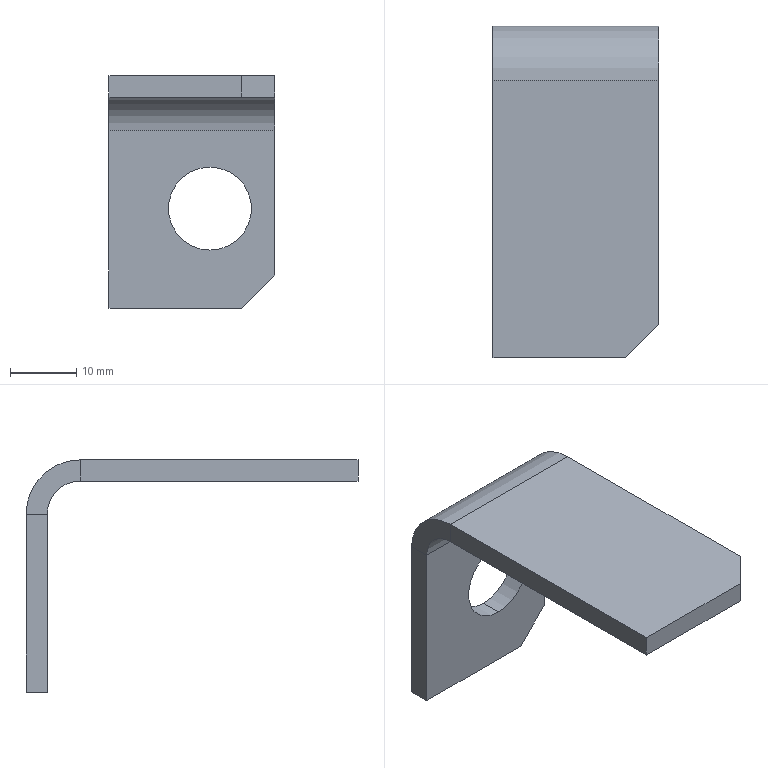Part | SolidWorks | features Chamfer 1, FlatPattern 1, ICE 1, SMBaseFlange 1, SheetMetal 1 | 1 solid | 18 faces | box 25 x 50 x 35 mm | volume 5845 mm3 | plane 14 | cylinder 4 | commonest cylinder face diameters 12.5 x2 10 x1 16.4 x1
STEP:
#1=CARTESIAN_POINT('',(15.2,46.8,-13.75));
#2=VERTEX_POINT('',#1);
#3=CARTESIAN_POINT('',(15.2,46.8,-26.25));
#4=VERTEX_POINT('',#3);
#5=CARTESIAN_POINT('',(15.2,46.8,-20.));
#6=DIRECTION('',(0.,-1.,0.));
#7=DIRECTION('',(0.,0.,1.));
#8=AXIS2_PLACEMENT_3D('',#5,#6,#7);
#9=CIRCLE('',#8,6.25);
#10=EDGE_CURVE('',#2,#4,#9,.T.);
#11=ORIENTED_EDGE('',*,*,#10,.T.);
#12=CARTESIAN_POINT('',(15.2,50.,-26.25));
#13=VERTEX_POINT('',#12);
#14=CARTESIAN_POINT('',(15.2,-0.001,-26.25));
#15=DIRECTION('',(0.,1.,0.));
#16=VECTOR('',#15,1000.);
#17=LINE('',#14,#16);
#18=EDGE_CURVE('',#4,#13,#17,.T.);
#19=ORIENTED_EDGE('',*,*,#18,.T.);
#20=CARTESIAN_POINT('',(15.2,50.,-13.75));
#21=VERTEX_POINT('',#20);
#22=CARTESIAN_POINT('',(15.2,50.,-20.));
#23=DIRECTION('',(0.,1.,0.));
#24=DIRECTION('',(0.,0.,1.));
#25=AXIS2_PLACEMENT_3D('',#22,#23,#24);
#26=CIRCLE('',#25,6.25);
#27=EDGE_CURVE('',#13,#21,#26,.T.);
#28=ORIENTED_EDGE('',*,*,#27,.T.);
#29=CARTESIAN_POINT('',(15.2,-0.001,-13.75));
#30=DIRECTION('',(0.,1.,0.));
#31=VECTOR('',#30,1000.);
#32=LINE('',#29,#31);
#33=EDGE_CURVE('',#2,#21,#32,.T.);
#34=ORIENTED_EDGE('',*,*,#33,.F.);
#35=EDGE_LOOP('',(#11,#19,#28,#34));
#36=FACE_OUTER_BOUND('',#35,.T.);
#37=CARTESIAN_POINT('',(15.2,-0.001,-20.));
#38=DIRECTION('',(0.,1.,0.));
#39=DIRECTION('',(0.,0.,1.));
#40=AXIS2_PLACEMENT_3D('',#37,#38,#39);
#41=CYLINDRICAL_SURFACE('',#40,6.25);
#42=ADVANCED_FACE('',(#36),#41,.F.);
#43=CARTESIAN_POINT('',(25.,50.,-8.2));
#44=VERTEX_POINT('',#43);
#45=CARTESIAN_POINT('',(25.,46.8,-8.2));
#46=VERTEX_POINT('',#45);
#47=CARTESIAN_POINT('',(25.,50.,-8.2));
#48=DIRECTION('',(0.,-1.,0.));
#49=VECTOR('',#48,1000.);
#50=LINE('',#47,#49);
#51=EDGE_CURVE('',#44,#46,#50,.T.);
#52=ORIENTED_EDGE('',*,*,#51,.F.);
#53=CARTESIAN_POINT('',(25.,41.8,0.));
#54=VERTEX_POINT('',#53);
#55=CARTESIAN_POINT('',(25.,41.8,-8.2));
#56=DIRECTION('',(-1.,0.,0.));
#57=DIRECTION('',(0.,0.,-1.));
#58=AXIS2_PLACEMENT_3D('',#55,#56,#57);
#59=CIRCLE('',#58,8.2);
#60=EDGE_CURVE('',#54,#44,#59,.T.);
#61=ORIENTED_EDGE('',*,*,#60,.F.);
#62=CARTESIAN_POINT('',(25.,41.8,-3.2));
#63=VERTEX_POINT('',#62);
#64=CARTESIAN_POINT('',(25.,41.8,-3.2));
#65=DIRECTION('',(0.,0.,1.));
#66=VECTOR('',#65,1000.);
#67=LINE('',#64,#66);
#68=EDGE_CURVE('',#63,#54,#67,.T.);
#69=ORIENTED_EDGE('',*,*,#68,.F.);
#70=CARTESIAN_POINT('',(25.,41.8,-8.2));
#71=DIRECTION('',(-1.,0.,0.));
#72=DIRECTION('',(0.,0.,-1.));
#73=AXIS2_PLACEMENT_3D('',#70,#71,#72);
#74=CIRCLE('',#73,5.);
#75=EDGE_CURVE('',#63,#46,#74,.T.);
#76=ORIENTED_EDGE('',*,*,#75,.T.);
#77=EDGE_LOOP('',(#52,#61,#69,#76));
#78=FACE_OUTER_BOUND('',#77,.T.);
#79=CARTESIAN_POINT('',(25.,50.,-8.2));
#80=DIRECTION('',(1.,0.,0.));
#81=DIRECTION('',(0.,0.,-1.));
#82=AXIS2_PLACEMENT_3D('',#79,#80,#81);
#83=PLANE('',#82);
#84=ADVANCED_FACE('',(#78),#83,.T.);
#85=CARTESIAN_POINT('',(25.,46.8,-30.));
#86=VERTEX_POINT('',#85);
#87=CARTESIAN_POINT('',(25.,46.8,0.));
#88=DIRECTION('',(0.,0.,-1.));
#89=VECTOR('',#88,1000.);
#90=LINE('',#87,#89);
#91=EDGE_CURVE('',#46,#86,#90,.T.);
#92=ORIENTED_EDGE('',*,*,#91,.T.);
#93=CARTESIAN_POINT('',(25.,50.,-30.));
#94=VERTEX_POINT('',#93);
#95=CARTESIAN_POINT('',(25.,41.8,-30.));
#96=DIRECTION('',(0.,1.,0.));
#97=VECTOR('',#96,1000.);
#98=LINE('',#95,#97);
#99=EDGE_CURVE('',#86,#94,#98,.T.);
#100=ORIENTED_EDGE('',*,*,#99,.T.);
#101=CARTESIAN_POINT('',(25.,50.,0.));
#102=DIRECTION('',(0.,0.,-1.));
#103=VECTOR('',#102,1000.);
#104=LINE('',#101,#103);
#105=EDGE_CURVE('',#44,#94,#104,.T.);
#106=ORIENTED_EDGE('',*,*,#105,.F.);
#107=ORIENTED_EDGE('',*,*,#51,.T.);
#108=EDGE_LOOP('',(#92,#100,#106,#107));
#109=FACE_OUTER_BOUND('',#108,.T.);
#110=CARTESIAN_POINT('',(25.,41.8,-3.2));
#111=DIRECTION('',(1.,0.,0.));
#112=DIRECTION('',(0.,0.,-1.));
#113=AXIS2_PLACEMENT_3D('',#110,#111,#112);
#114=PLANE('',#113);
#115=ADVANCED_FACE('',(#109),#114,.T.);
#116=CARTESIAN_POINT('',(0.,41.8,0.));
#117=VERTEX_POINT('',#116);
#118=CARTESIAN_POINT('',(0.,41.8,-3.2));
#119=VERTEX_POINT('',#118);
#120=CARTESIAN_POINT('',(0.,41.8,0.));
#121=DIRECTION('',(0.,0.,-1.));
#122=VECTOR('',#121,1000.);
#123=LINE('',#120,#122);
#124=EDGE_CURVE('',#117,#119,#123,.T.);
#125=ORIENTED_EDGE('',*,*,#124,.F.);
#126=CARTESIAN_POINT('',(0.,50.,-8.2));
#127=VERTEX_POINT('',#126);
#128=CARTESIAN_POINT('',(0.,41.8,-8.2));
#129=DIRECTION('',(-1.,0.,0.));
#130=DIRECTION('',(0.,0.,-1.));
#131=AXIS2_PLACEMENT_3D('',#128,#129,#130);
#132=CIRCLE('',#131,8.2);
#133=EDGE_CURVE('',#117,#127,#132,.T.);
#134=ORIENTED_EDGE('',*,*,#133,.T.);
#135=CARTESIAN_POINT('',(0.,46.8,-8.2));
#136=VERTEX_POINT('',#135);
#137=CARTESIAN_POINT('',(0.,46.8,-8.2));
#138=DIRECTION('',(0.,1.,0.));
#139=VECTOR('',#138,1000.);
#140=LINE('',#137,#139);
#141=EDGE_CURVE('',#136,#127,#140,.T.);
#142=ORIENTED_EDGE('',*,*,#141,.F.);
#143=CARTESIAN_POINT('',(0.,41.8,-8.2));
#144=DIRECTION('',(-1.,0.,0.));
#145=DIRECTION('',(0.,0.,-1.));
#146=AXIS2_PLACEMENT_3D('',#143,#144,#145);
#147=CIRCLE('',#146,5.);
#148=EDGE_CURVE('',#119,#136,#147,.T.);
#149=ORIENTED_EDGE('',*,*,#148,.F.);
#150=EDGE_LOOP('',(#125,#134,#142,#149));
#151=FACE_OUTER_BOUND('',#150,.T.);
#152=CARTESIAN_POINT('',(0.,41.8,0.));
#153=DIRECTION('',(-1.,0.,0.));
#154=DIRECTION('',(0.,0.,1.));
#155=AXIS2_PLACEMENT_3D('',#152,#153,#154);
#156=PLANE('',#155);
#157=ADVANCED_FACE('',(#151),#156,.T.);
#158=CARTESIAN_POINT('',(0.,0.,0.));
#159=VERTEX_POINT('',#158);
#160=CARTESIAN_POINT('',(0.,0.,0.));
#161=DIRECTION('',(0.,1.,0.));
#162=VECTOR('',#161,1000.);
#163=LINE('',#160,#162);
#164=EDGE_CURVE('',#159,#117,#163,.T.);
#165=ORIENTED_EDGE('',*,*,#164,.T.);
#166=ORIENTED_EDGE('',*,*,#124,.T.);
#167=CARTESIAN_POINT('',(0.,0.,-3.2));
#168=VERTEX_POINT('',#167);
#169=CARTESIAN_POINT('',(0.,0.,-3.2));
#170=DIRECTION('',(0.,1.,0.));
#171=VECTOR('',#170,1000.);
#172=LINE('',#169,#171);
#173=EDGE_CURVE('',#168,#119,#172,.T.);
#174=ORIENTED_EDGE('',*,*,#173,.F.);
#175=CARTESIAN_POINT('',(0.,0.,-3.2));
#176=DIRECTION('',(0.,0.,1.));
#177=VECTOR('',#176,1000.);
#178=LINE('',#175,#177);
#179=EDGE_CURVE('',#168,#159,#178,.T.);
#180=ORIENTED_EDGE('',*,*,#179,.T.);
#181=EDGE_LOOP('',(#165,#166,#174,#180));
#182=FACE_OUTER_BOUND('',#181,.T.);
#183=CARTESIAN_POINT('',(0.,46.8,-8.2));
#184=DIRECTION('',(-1.,0.,0.));
#185=DIRECTION('',(0.,0.,1.));
#186=AXIS2_PLACEMENT_3D('',#183,#184,#185);
#187=PLANE('',#186);
#188=ADVANCED_FACE('',(#182),#187,.T.);
#189=ORIENTED_EDGE('',*,*,#10,.F.);
#190=CARTESIAN_POINT('',(15.2,46.8,-20.));
#191=DIRECTION('',(0.,-1.,0.));
#192=DIRECTION('',(0.,0.,1.));
#193=AXIS2_PLACEMENT_3D('',#190,#191,#192);
#194=CIRCLE('',#193,6.25);
#195=EDGE_CURVE('',#4,#2,#194,.T.);
#196=ORIENTED_EDGE('',*,*,#195,.F.);
#197=EDGE_LOOP('',(#189,#196));
#198=FACE_BOUND('',#197,.T.);
#199=CARTESIAN_POINT('',(20.,46.8,-35.));
#200=VERTEX_POINT('',#199);
#201=CARTESIAN_POINT('',(0.,46.8,-35.));
#202=VERTEX_POINT('',#201);
#203=CARTESIAN_POINT('',(25.,46.8,-35.));
#204=DIRECTION('',(-1.,0.,0.));
#205=VECTOR('',#204,1000.);
#206=LINE('',#203,#205);
#207=EDGE_CURVE('',#200,#202,#206,.T.);
#208=ORIENTED_EDGE('',*,*,#207,.F.);
#209=CARTESIAN_POINT('',(20.,46.8,-35.));
#210=DIRECTION('',(0.7071,0.,0.7071));
#211=VECTOR('',#210,1000.);
#212=LINE('',#209,#211);
#213=EDGE_CURVE('',#200,#86,#212,.T.);
#214=ORIENTED_EDGE('',*,*,#213,.T.);
#215=ORIENTED_EDGE('',*,*,#91,.F.);
#216=CARTESIAN_POINT('',(25.,46.8,-8.2));
#217=DIRECTION('',(-1.,0.,0.));
#218=VECTOR('',#217,1000.);
#219=LINE('',#216,#218);
#220=EDGE_CURVE('',#46,#136,#219,.T.);
#221=ORIENTED_EDGE('',*,*,#220,.T.);
#222=CARTESIAN_POINT('',(0.,46.8,0.));
#223=DIRECTION('',(0.,0.,-1.));
#224=VECTOR('',#223,1000.);
#225=LINE('',#222,#224);
#226=EDGE_CURVE('',#136,#202,#225,.T.);
#227=ORIENTED_EDGE('',*,*,#226,.T.);
#228=EDGE_LOOP('',(#208,#214,#215,#221,#227));
#229=FACE_OUTER_BOUND('',#228,.T.);
#230=CARTESIAN_POINT('',(25.,46.8,0.));
#231=DIRECTION('',(0.,1.,0.));
#232=DIRECTION('',(0.,0.,1.));
#233=AXIS2_PLACEMENT_3D('',#230,#231,#232);
#234=PLANE('',#233);
#235=ADVANCED_FACE('',(#198,#229),#234,.F.);
#236=CARTESIAN_POINT('',(20.,50.,-35.));
#237=VERTEX_POINT('',#236);
#238=CARTESIAN_POINT('',(0.,50.,-35.));
#239=VERTEX_POINT('',#238);
#240=CARTESIAN_POINT('',(25.,50.,-35.));
#241=DIRECTION('',(-1.,0.,0.));
#242=VECTOR('',#241,1000.);
#243=LINE('',#240,#242);
#244=EDGE_CURVE('',#237,#239,#243,.T.);
#245=ORIENTED_EDGE('',*,*,#244,.F.);
#246=CARTESIAN_POINT('',(20.,50.,-35.));
#247=DIRECTION('',(0.,-1.,0.));
#248=VECTOR('',#247,1000.);
#249=LINE('',#246,#248);
#250=EDGE_CURVE('',#237,#200,#249,.T.);
#251=ORIENTED_EDGE('',*,*,#250,.T.);
#252=ORIENTED_EDGE('',*,*,#207,.T.);
#253=CARTESIAN_POINT('',(0.,50.,-35.));
#254=DIRECTION('',(0.,-1.,0.));
#255=VECTOR('',#254,1000.);
#256=LINE('',#253,#255);
#257=EDGE_CURVE('',#239,#202,#256,.T.);
#258=ORIENTED_EDGE('',*,*,#257,.F.);
#259=EDGE_LOOP('',(#245,#251,#252,#258));
#260=FACE_OUTER_BOUND('',#259,.T.);
#261=CARTESIAN_POINT('',(25.,50.,-35.));
#262=DIRECTION('',(0.,0.,-1.));
#263=DIRECTION('',(-1.,0.,0.));
#264=AXIS2_PLACEMENT_3D('',#261,#262,#263);
#265=PLANE('',#264);
#266=ADVANCED_FACE('',(#260),#265,.T.);
#267=CARTESIAN_POINT('',(15.2,50.,-20.));
#268=DIRECTION('',(0.,1.,0.));
#269=DIRECTION('',(0.,0.,1.));
#270=AXIS2_PLACEMENT_3D('',#267,#268,#269);
#271=CIRCLE('',#270,6.25);
#272=EDGE_CURVE('',#21,#13,#271,.T.);
#273=ORIENTED_EDGE('',*,*,#272,.F.);
#274=ORIENTED_EDGE('',*,*,#27,.F.);
#275=EDGE_LOOP('',(#273,#274));
#276=FACE_BOUND('',#275,.T.);
#277=ORIENTED_EDGE('',*,*,#105,.T.);
#278=CARTESIAN_POINT('',(40.,50.,-15.));
#279=DIRECTION('',(-0.7071,0.,-0.7071));
#280=VECTOR('',#279,1000.);
#281=LINE('',#278,#280);
#282=EDGE_CURVE('',#94,#237,#281,.T.);
#283=ORIENTED_EDGE('',*,*,#282,.T.);
#284=ORIENTED_EDGE('',*,*,#244,.T.);
#285=CARTESIAN_POINT('',(0.,50.,0.));
#286=DIRECTION('',(0.,0.,-1.));
#287=VECTOR('',#286,1000.);
#288=LINE('',#285,#287);
#289=EDGE_CURVE('',#127,#239,#288,.T.);
#290=ORIENTED_EDGE('',*,*,#289,.F.);
#291=CARTESIAN_POINT('',(25.,50.,-8.2));
#292=DIRECTION('',(-1.,0.,0.));
#293=VECTOR('',#292,1000.);
#294=LINE('',#291,#293);
#295=EDGE_CURVE('',#44,#127,#294,.T.);
#296=ORIENTED_EDGE('',*,*,#295,.F.);
#297=EDGE_LOOP('',(#277,#283,#284,#290,#296));
#298=FACE_OUTER_BOUND('',#297,.T.);
#299=CARTESIAN_POINT('',(25.,50.,0.));
#300=DIRECTION('',(0.,1.,0.));
#301=DIRECTION('',(0.,0.,1.));
#302=AXIS2_PLACEMENT_3D('',#299,#300,#301);
#303=PLANE('',#302);
#304=ADVANCED_FACE('',(#276,#298),#303,.T.);
#305=ORIENTED_EDGE('',*,*,#133,.F.);
#306=CARTESIAN_POINT('',(25.,41.8,0.));
#307=DIRECTION('',(-1.,0.,0.));
#308=VECTOR('',#307,1000.);
#309=LINE('',#306,#308);
#310=EDGE_CURVE('',#54,#117,#309,.T.);
#311=ORIENTED_EDGE('',*,*,#310,.F.);
#312=ORIENTED_EDGE('',*,*,#60,.T.);
#313=ORIENTED_EDGE('',*,*,#295,.T.);
#314=EDGE_LOOP('',(#305,#311,#312,#313));
#315=FACE_OUTER_BOUND('',#314,.T.);
#316=CARTESIAN_POINT('',(25.,41.8,-8.2));
#317=DIRECTION('',(-1.,0.,0.));
#318=DIRECTION('',(0.,0.,1.));
#319=AXIS2_PLACEMENT_3D('',#316,#317,#318);
#320=CYLINDRICAL_SURFACE('',#319,8.2);
#321=ADVANCED_FACE('',(#315),#320,.T.);
#322=CARTESIAN_POINT('',(20.,0.,0.));
#323=VERTEX_POINT('',#322);
#324=CARTESIAN_POINT('',(25.,0.,0.));
#325=DIRECTION('',(-1.,0.,0.));
#326=VECTOR('',#325,1000.);
#327=LINE('',#324,#326);
#328=EDGE_CURVE('',#323,#159,#327,.T.);
#329=ORIENTED_EDGE('',*,*,#328,.F.);
#330=CARTESIAN_POINT('',(25.,5.,0.));
#331=VERTEX_POINT('',#330);
#332=CARTESIAN_POINT('',(22.5,2.5,0.));
#333=DIRECTION('',(0.7071,0.7071,0.));
#334=VECTOR('',#333,1000.);
#335=LINE('',#332,#334);
#336=EDGE_CURVE('',#323,#331,#335,.T.);
#337=ORIENTED_EDGE('',*,*,#336,.T.);
#338=CARTESIAN_POINT('',(25.,0.,0.));
#339=DIRECTION('',(0.,1.,0.));
#340=VECTOR('',#339,1000.);
#341=LINE('',#338,#340);
#342=EDGE_CURVE('',#331,#54,#341,.T.);
#343=ORIENTED_EDGE('',*,*,#342,.T.);
#344=ORIENTED_EDGE('',*,*,#310,.T.);
#345=ORIENTED_EDGE('',*,*,#164,.F.);
#346=EDGE_LOOP('',(#329,#337,#343,#344,#345));
#347=FACE_OUTER_BOUND('',#346,.T.);
#348=CARTESIAN_POINT('',(25.,0.,0.));
#349=DIRECTION('',(0.,0.,1.));
#350=DIRECTION('',(1.,0.,0.));
#351=AXIS2_PLACEMENT_3D('',#348,#349,#350);
#352=PLANE('',#351);
#353=ADVANCED_FACE('',(#347),#352,.T.);
#354=CARTESIAN_POINT('',(20.,0.,-3.2));
#355=VERTEX_POINT('',#354);
#356=CARTESIAN_POINT('',(25.,0.,-3.2));
#357=DIRECTION('',(-1.,0.,0.));
#358=VECTOR('',#357,1000.);
#359=LINE('',#356,#358);
#360=EDGE_CURVE('',#355,#168,#359,.T.);
#361=ORIENTED_EDGE('',*,*,#360,.F.);
#362=CARTESIAN_POINT('',(20.,0.,-3.2));
#363=DIRECTION('',(0.,0.,1.));
#364=VECTOR('',#363,1000.);
#365=LINE('',#362,#364);
#366=EDGE_CURVE('',#355,#323,#365,.T.);
#367=ORIENTED_EDGE('',*,*,#366,.T.);
#368=ORIENTED_EDGE('',*,*,#328,.T.);
#369=ORIENTED_EDGE('',*,*,#179,.F.);
#370=EDGE_LOOP('',(#361,#367,#368,#369));
#371=FACE_OUTER_BOUND('',#370,.T.);
#372=CARTESIAN_POINT('',(25.,0.,-3.2));
#373=DIRECTION('',(0.,-1.,0.));
#374=DIRECTION('',(0.,0.,-1.));
#375=AXIS2_PLACEMENT_3D('',#372,#373,#374);
#376=PLANE('',#375);
#377=ADVANCED_FACE('',(#371),#376,.T.);
#378=CARTESIAN_POINT('',(25.,5.,-3.2));
#379=VERTEX_POINT('',#378);
#380=CARTESIAN_POINT('',(25.,0.,-3.2));
#381=DIRECTION('',(0.,1.,0.));
#382=VECTOR('',#381,1000.);
#383=LINE('',#380,#382);
#384=EDGE_CURVE('',#379,#63,#383,.T.);
#385=ORIENTED_EDGE('',*,*,#384,.F.);
#386=CARTESIAN_POINT('',(20.,0.,-3.2));
#387=DIRECTION('',(-0.7071,-0.7071,0.));
#388=VECTOR('',#387,1000.);
#389=LINE('',#386,#388);
#390=EDGE_CURVE('',#379,#355,#389,.T.);
#391=ORIENTED_EDGE('',*,*,#390,.T.);
#392=ORIENTED_EDGE('',*,*,#360,.T.);
#393=ORIENTED_EDGE('',*,*,#173,.T.);
#394=CARTESIAN_POINT('',(25.,41.8,-3.2));
#395=DIRECTION('',(-1.,0.,0.));
#396=VECTOR('',#395,1000.);
#397=LINE('',#394,#396);
#398=EDGE_CURVE('',#63,#119,#397,.T.);
#399=ORIENTED_EDGE('',*,*,#398,.F.);
#400=EDGE_LOOP('',(#385,#391,#392,#393,#399));
#401=FACE_OUTER_BOUND('',#400,.T.);
#402=CARTESIAN_POINT('',(25.,0.,-3.2));
#403=DIRECTION('',(0.,0.,1.));
#404=DIRECTION('',(1.,0.,0.));
#405=AXIS2_PLACEMENT_3D('',#402,#403,#404);
#406=PLANE('',#405);
#407=ADVANCED_FACE('',(#401),#406,.F.);
#408=ORIENTED_EDGE('',*,*,#148,.T.);
#409=ORIENTED_EDGE('',*,*,#220,.F.);
#410=ORIENTED_EDGE('',*,*,#75,.F.);
#411=ORIENTED_EDGE('',*,*,#398,.T.);
#412=EDGE_LOOP('',(#408,#409,#410,#411));
#413=FACE_OUTER_BOUND('',#412,.T.);
#414=CARTESIAN_POINT('',(25.,41.8,-8.2));
#415=DIRECTION('',(-1.,0.,0.));
#416=DIRECTION('',(0.,0.,1.));
#417=AXIS2_PLACEMENT_3D('',#414,#415,#416);
#418=CYLINDRICAL_SURFACE('',#417,5.);
#419=ADVANCED_FACE('',(#413),#418,.F.);
#420=ORIENTED_EDGE('',*,*,#342,.F.);
#421=CARTESIAN_POINT('',(25.,5.,-8.2));
#422=DIRECTION('',(0.,0.,-1.));
#423=VECTOR('',#422,1000.);
#424=LINE('',#421,#423);
#425=EDGE_CURVE('',#331,#379,#424,.T.);
#426=ORIENTED_EDGE('',*,*,#425,.T.);
#427=ORIENTED_EDGE('',*,*,#384,.T.);
#428=ORIENTED_EDGE('',*,*,#68,.T.);
#429=EDGE_LOOP('',(#420,#426,#427,#428));
#430=FACE_OUTER_BOUND('',#429,.T.);
#431=CARTESIAN_POINT('',(25.,41.8,-8.2));
#432=DIRECTION('',(1.,0.,0.));
#433=DIRECTION('',(0.,0.,-1.));
#434=AXIS2_PLACEMENT_3D('',#431,#432,#433);
#435=PLANE('',#434);
#436=ADVANCED_FACE('',(#430),#435,.T.);
#437=ORIENTED_EDGE('',*,*,#226,.F.);
#438=ORIENTED_EDGE('',*,*,#141,.T.);
#439=ORIENTED_EDGE('',*,*,#289,.T.);
#440=ORIENTED_EDGE('',*,*,#257,.T.);
#441=EDGE_LOOP('',(#437,#438,#439,#440));
#442=FACE_OUTER_BOUND('',#441,.T.);
#443=CARTESIAN_POINT('',(0.,41.8,-8.2));
#444=DIRECTION('',(1.,0.,0.));
#445=DIRECTION('',(0.,0.,-1.));
#446=AXIS2_PLACEMENT_3D('',#443,#444,#445);
#447=PLANE('',#446);
#448=ADVANCED_FACE('',(#442),#447,.F.);
#449=ORIENTED_EDGE('',*,*,#18,.F.);
#450=ORIENTED_EDGE('',*,*,#195,.T.);
#451=ORIENTED_EDGE('',*,*,#33,.T.);
#452=ORIENTED_EDGE('',*,*,#272,.T.);
#453=EDGE_LOOP('',(#449,#450,#451,#452));
#454=FACE_OUTER_BOUND('',#453,.T.);
#455=CARTESIAN_POINT('',(15.2,-0.001,-20.));
#456=DIRECTION('',(0.,1.,0.));
#457=DIRECTION('',(0.,0.,1.));
#458=AXIS2_PLACEMENT_3D('',#455,#456,#457);
#459=CYLINDRICAL_SURFACE('',#458,6.25);
#460=ADVANCED_FACE('',(#454),#459,.F.);
#461=ORIENTED_EDGE('',*,*,#282,.F.);
#462=ORIENTED_EDGE('',*,*,#99,.F.);
#463=ORIENTED_EDGE('',*,*,#213,.F.);
#464=ORIENTED_EDGE('',*,*,#250,.F.);
#465=EDGE_LOOP('',(#461,#462,#463,#464));
#466=FACE_OUTER_BOUND('',#465,.T.);
#467=CARTESIAN_POINT('',(20.,50.,-35.));
#468=DIRECTION('',(-0.7071,0.,0.7071));
#469=DIRECTION('',(0.,-1.,0.));
#470=AXIS2_PLACEMENT_3D('',#467,#468,#469);
#471=PLANE('',#470);
#472=ADVANCED_FACE('',(#466),#471,.F.);
#473=ORIENTED_EDGE('',*,*,#390,.F.);
#474=ORIENTED_EDGE('',*,*,#425,.F.);
#475=ORIENTED_EDGE('',*,*,#336,.F.);
#476=ORIENTED_EDGE('',*,*,#366,.F.);
#477=EDGE_LOOP('',(#473,#474,#475,#476));
#478=FACE_OUTER_BOUND('',#477,.T.);
#479=CARTESIAN_POINT('',(20.,0.,-3.2));
#480=DIRECTION('',(-0.7071,0.7071,0.));
#481=DIRECTION('',(0.,0.,1.));
#482=AXIS2_PLACEMENT_3D('',#479,#480,#481);
#483=PLANE('',#482);
#484=ADVANCED_FACE('',(#478),#483,.F.);
#485=CLOSED_SHELL('',(#42,#84,#115,#157,#188,#235,#266,#304,#321,#353,#377,#407,#419,#436,#448,#460,#472,#484));
#486=MANIFOLD_SOLID_BREP('',#485);
#487=CARTESIAN_POINT('',(0.,0.,0.));
#488=DIRECTION('',(0.,0.,1.));
#489=DIRECTION('',(1.,0.,0.));
#490=AXIS2_PLACEMENT_3D('',#487,#488,#489);
#491=(LENGTH_UNIT()NAMED_UNIT(*)SI_UNIT(.MILLI.,.METRE.));
#492=UNCERTAINTY_MEASURE_WITH_UNIT(LENGTH_MEASURE(0.00001),#491,'','');
#493=(NAMED_UNIT(*)PLANE_ANGLE_UNIT()SI_UNIT($,.RADIAN.));
#494=(NAMED_UNIT(*)SI_UNIT($,.STERADIAN.)SOLID_ANGLE_UNIT());
#495=(GEOMETRIC_REPRESENTATION_CONTEXT(3)GLOBAL_UNCERTAINTY_ASSIGNED_CONTEXT((#492))GLOBAL_UNIT_ASSIGNED_CONTEXT((#491,#493,#494))REPRESENTATION_CONTEXT('',''));
#496=ADVANCED_BREP_SHAPE_REPRESENTATION('',(#486,#490),#495);